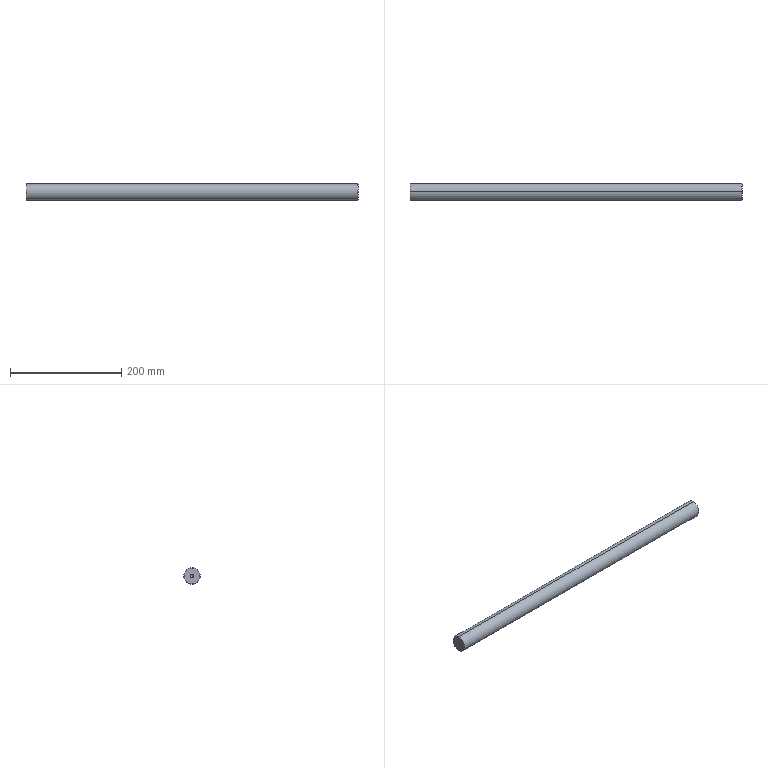Part | STEP file | 001-004-SCD11_D30_L598_M6 | 1 solid | 14 faces | box 598 x 30 x 30 mm | volume 422409 mm3 | cone 8 | cylinder 4 | plane 2 | commonest cylinder face diameters 4.917 x2 30 x2
STEP:
#1=CARTESIAN_POINT('',(0.,0.,0.));
#2=DIRECTION('',(0.,0.,1.));
#3=DIRECTION('',(1.,0.,0.));
#4=AXIS2_PLACEMENT_3D('',#1,#2,#3);
#5=CARTESIAN_POINT('',(598.,0.,14.293));
#6=VERTEX_POINT('',#5);
#7=CARTESIAN_POINT('',(598.,0.,-14.293));
#8=VERTEX_POINT('',#7);
#9=CARTESIAN_POINT('',(598.,0.,0.));
#10=DIRECTION('',(-1.,0.,0.));
#11=DIRECTION('',(0.,0.,1.));
#12=AXIS2_PLACEMENT_3D('',#9,#10,#11);
#13=CIRCLE('',#12,14.293);
#14=CARTESIAN_POINT('',(598.,0.,0.));
#15=DIRECTION('',(-1.,0.,0.));
#16=DIRECTION('',(0.,0.,1.));
#17=AXIS2_PLACEMENT_3D('',#14,#15,#16);
#18=CONICAL_SURFACE('',#17,14.293,0.7854);
#19=CARTESIAN_POINT('',(0.,0.));
#20=DIRECTION('',(1.,0.));
#21=VECTOR('',#20,1.);
#22=LINE('',#19,#21);
#23=(GEOMETRIC_REPRESENTATION_CONTEXT(2)PARAMETRIC_REPRESENTATION_CONTEXT()REPRESENTATION_CONTEXT('',''));
#24=DEFINITIONAL_REPRESENTATION('',(#22),#23);
#25=PCURVE('',#18,#24);
#26=CARTESIAN_POINT('',(598.,14.293,0.));
#27=DIRECTION('',(-1.,0.,0.));
#28=DIRECTION('',(0.,0.,1.));
#29=AXIS2_PLACEMENT_3D('',#26,#27,#28);
#30=PLANE('',#29);
#31=CARTESIAN_POINT('',(0.,-14.293));
#32=DIRECTION('',(1.,0.));
#33=AXIS2_PLACEMENT_2D('',#31,#32);
#34=CIRCLE('',#33,14.293);
#35=(GEOMETRIC_REPRESENTATION_CONTEXT(2)PARAMETRIC_REPRESENTATION_CONTEXT()REPRESENTATION_CONTEXT('',''));
#36=DEFINITIONAL_REPRESENTATION('',(#34),#35);
#37=PCURVE('',#30,#36);
#38=SURFACE_CURVE('',#13,(#25,#37),.PCURVE_S1.);
#39=EDGE_CURVE('',#6,#8,#38,.T.);
#40=ORIENTED_EDGE('',*,*,#39,.T.);
#41=CARTESIAN_POINT('',(597.293,0.,-15.));
#42=VERTEX_POINT('',#41);
#43=CARTESIAN_POINT('',(598.,0.,-14.293));
#44=DIRECTION('',(-0.7071,0.,-0.7071));
#45=VECTOR('',#44,1.);
#46=LINE('',#43,#45);
#47=CARTESIAN_POINT('',(3.142,0.));
#48=DIRECTION('',(0.,1.));
#49=VECTOR('',#48,1.);
#50=LINE('',#47,#49);
#51=(GEOMETRIC_REPRESENTATION_CONTEXT(2)PARAMETRIC_REPRESENTATION_CONTEXT()REPRESENTATION_CONTEXT('',''));
#52=DEFINITIONAL_REPRESENTATION('',(#50),#51);
#53=PCURVE('',#18,#52);
#54=CARTESIAN_POINT('',(598.,0.,0.));
#55=DIRECTION('',(-1.,0.,0.));
#56=DIRECTION('',(0.,0.,1.));
#57=AXIS2_PLACEMENT_3D('',#54,#55,#56);
#58=CONICAL_SURFACE('',#57,14.293,0.7854);
#59=CARTESIAN_POINT('',(3.142,0.));
#60=DIRECTION('',(0.,1.));
#61=VECTOR('',#60,1.);
#62=LINE('',#59,#61);
#63=(GEOMETRIC_REPRESENTATION_CONTEXT(2)PARAMETRIC_REPRESENTATION_CONTEXT()REPRESENTATION_CONTEXT('',''));
#64=DEFINITIONAL_REPRESENTATION('',(#62),#63);
#65=PCURVE('',#58,#64);
#66=SURFACE_CURVE('',#46,(#53,#65),.PCURVE_S1.);
#67=EDGE_CURVE('',#8,#42,#66,.T.);
#68=ORIENTED_EDGE('',*,*,#67,.T.);
#69=CARTESIAN_POINT('',(597.293,0.,15.));
#70=VERTEX_POINT('',#69);
#71=CARTESIAN_POINT('',(597.293,0.,0.));
#72=DIRECTION('',(-1.,0.,0.));
#73=DIRECTION('',(0.,0.,1.));
#74=AXIS2_PLACEMENT_3D('',#71,#72,#73);
#75=CIRCLE('',#74,15.);
#76=CARTESIAN_POINT('',(0.,0.7071));
#77=DIRECTION('',(1.,0.));
#78=VECTOR('',#77,1.);
#79=LINE('',#76,#78);
#80=(GEOMETRIC_REPRESENTATION_CONTEXT(2)PARAMETRIC_REPRESENTATION_CONTEXT()REPRESENTATION_CONTEXT('',''));
#81=DEFINITIONAL_REPRESENTATION('',(#79),#80);
#82=PCURVE('',#18,#81);
#83=CARTESIAN_POINT('',(598.,0.,0.));
#84=DIRECTION('',(-1.,0.,0.));
#85=DIRECTION('',(0.,0.,1.));
#86=AXIS2_PLACEMENT_3D('',#83,#84,#85);
#87=CYLINDRICAL_SURFACE('',#86,15.);
#88=CARTESIAN_POINT('',(0.,0.7071));
#89=DIRECTION('',(1.,0.));
#90=VECTOR('',#89,1.);
#91=LINE('',#88,#90);
#92=(GEOMETRIC_REPRESENTATION_CONTEXT(2)PARAMETRIC_REPRESENTATION_CONTEXT()REPRESENTATION_CONTEXT('',''));
#93=DEFINITIONAL_REPRESENTATION('',(#91),#92);
#94=PCURVE('',#87,#93);
#95=SURFACE_CURVE('',#75,(#82,#94),.PCURVE_S1.);
#96=EDGE_CURVE('',#70,#42,#95,.T.);
#97=ORIENTED_EDGE('',*,*,#96,.F.);
#98=CARTESIAN_POINT('',(598.,0.,14.293));
#99=DIRECTION('',(-0.7071,0.,0.7071));
#100=VECTOR('',#99,1.);
#101=LINE('',#98,#100);
#102=CARTESIAN_POINT('',(0.,0.));
#103=DIRECTION('',(0.,1.));
#104=VECTOR('',#103,1.);
#105=LINE('',#102,#104);
#106=(GEOMETRIC_REPRESENTATION_CONTEXT(2)PARAMETRIC_REPRESENTATION_CONTEXT()REPRESENTATION_CONTEXT('',''));
#107=DEFINITIONAL_REPRESENTATION('',(#105),#106);
#108=PCURVE('',#18,#107);
#109=CARTESIAN_POINT('',(6.283,0.));
#110=DIRECTION('',(0.,1.));
#111=VECTOR('',#110,1.);
#112=LINE('',#109,#111);
#113=(GEOMETRIC_REPRESENTATION_CONTEXT(2)PARAMETRIC_REPRESENTATION_CONTEXT()REPRESENTATION_CONTEXT('',''));
#114=DEFINITIONAL_REPRESENTATION('',(#112),#113);
#115=PCURVE('',#58,#114);
#116=SURFACE_CURVE('',#101,(#108,#115),.PCURVE_S1.);
#117=EDGE_CURVE('',#6,#70,#116,.T.);
#118=ORIENTED_EDGE('',*,*,#117,.F.);
#119=EDGE_LOOP('',(#40,#68,#97,#118));
#120=FACE_BOUND('',#119,.T.);
#121=ADVANCED_FACE('',(#120),#18,.T.);
#122=ORIENTED_EDGE('',*,*,#96,.T.);
#123=CARTESIAN_POINT('',(0.7071,0.,-15.));
#124=VERTEX_POINT('',#123);
#125=CARTESIAN_POINT('',(598.,0.,-15.));
#126=DIRECTION('',(-1.,0.,0.));
#127=VECTOR('',#126,1.);
#128=LINE('',#125,#127);
#129=CARTESIAN_POINT('',(3.142,0.));
#130=DIRECTION('',(0.,1.));
#131=VECTOR('',#130,1.);
#132=LINE('',#129,#131);
#133=(GEOMETRIC_REPRESENTATION_CONTEXT(2)PARAMETRIC_REPRESENTATION_CONTEXT()REPRESENTATION_CONTEXT('',''));
#134=DEFINITIONAL_REPRESENTATION('',(#132),#133);
#135=PCURVE('',#87,#134);
#136=CARTESIAN_POINT('',(598.,0.,0.));
#137=DIRECTION('',(-1.,0.,0.));
#138=DIRECTION('',(0.,0.,1.));
#139=AXIS2_PLACEMENT_3D('',#136,#137,#138);
#140=CYLINDRICAL_SURFACE('',#139,15.);
#141=CARTESIAN_POINT('',(3.142,0.));
#142=DIRECTION('',(0.,1.));
#143=VECTOR('',#142,1.);
#144=LINE('',#141,#143);
#145=(GEOMETRIC_REPRESENTATION_CONTEXT(2)PARAMETRIC_REPRESENTATION_CONTEXT()REPRESENTATION_CONTEXT('',''));
#146=DEFINITIONAL_REPRESENTATION('',(#144),#145);
#147=PCURVE('',#140,#146);
#148=SURFACE_CURVE('',#128,(#135,#147),.PCURVE_S1.);
#149=EDGE_CURVE('',#42,#124,#148,.T.);
#150=ORIENTED_EDGE('',*,*,#149,.T.);
#151=CARTESIAN_POINT('',(0.7071,0.,15.));
#152=VERTEX_POINT('',#151);
#153=CARTESIAN_POINT('',(0.7071,0.,0.));
#154=DIRECTION('',(-1.,0.,0.));
#155=DIRECTION('',(0.,0.,1.));
#156=AXIS2_PLACEMENT_3D('',#153,#154,#155);
#157=CIRCLE('',#156,15.);
#158=CARTESIAN_POINT('',(0.,597.293));
#159=DIRECTION('',(1.,0.));
#160=VECTOR('',#159,1.);
#161=LINE('',#158,#160);
#162=(GEOMETRIC_REPRESENTATION_CONTEXT(2)PARAMETRIC_REPRESENTATION_CONTEXT()REPRESENTATION_CONTEXT('',''));
#163=DEFINITIONAL_REPRESENTATION('',(#161),#162);
#164=PCURVE('',#87,#163);
#165=CARTESIAN_POINT('',(0.7071,0.,0.));
#166=DIRECTION('',(1.,0.,0.));
#167=DIRECTION('',(0.,0.,-1.));
#168=AXIS2_PLACEMENT_3D('',#165,#166,#167);
#169=CONICAL_SURFACE('',#168,15.,0.7854);
#170=CARTESIAN_POINT('',(3.142,0.));
#171=DIRECTION('',(-1.,0.));
#172=VECTOR('',#171,1.);
#173=LINE('',#170,#172);
#174=(GEOMETRIC_REPRESENTATION_CONTEXT(2)PARAMETRIC_REPRESENTATION_CONTEXT()REPRESENTATION_CONTEXT('',''));
#175=DEFINITIONAL_REPRESENTATION('',(#173),#174);
#176=PCURVE('',#169,#175);
#177=SURFACE_CURVE('',#157,(#164,#176),.PCURVE_S1.);
#178=EDGE_CURVE('',#152,#124,#177,.T.);
#179=ORIENTED_EDGE('',*,*,#178,.F.);
#180=CARTESIAN_POINT('',(598.,0.,15.));
#181=DIRECTION('',(-1.,0.,0.));
#182=VECTOR('',#181,1.);
#183=LINE('',#180,#182);
#184=CARTESIAN_POINT('',(0.,0.));
#185=DIRECTION('',(0.,1.));
#186=VECTOR('',#185,1.);
#187=LINE('',#184,#186);
#188=(GEOMETRIC_REPRESENTATION_CONTEXT(2)PARAMETRIC_REPRESENTATION_CONTEXT()REPRESENTATION_CONTEXT('',''));
#189=DEFINITIONAL_REPRESENTATION('',(#187),#188);
#190=PCURVE('',#87,#189);
#191=CARTESIAN_POINT('',(6.283,0.));
#192=DIRECTION('',(0.,1.));
#193=VECTOR('',#192,1.);
#194=LINE('',#191,#193);
#195=(GEOMETRIC_REPRESENTATION_CONTEXT(2)PARAMETRIC_REPRESENTATION_CONTEXT()REPRESENTATION_CONTEXT('',''));
#196=DEFINITIONAL_REPRESENTATION('',(#194),#195);
#197=PCURVE('',#140,#196);
#198=SURFACE_CURVE('',#183,(#190,#197),.PCURVE_S1.);
#199=EDGE_CURVE('',#70,#152,#198,.T.);
#200=ORIENTED_EDGE('',*,*,#199,.F.);
#201=EDGE_LOOP('',(#122,#150,#179,#200));
#202=FACE_BOUND('',#201,.T.);
#203=ADVANCED_FACE('',(#202),#87,.T.);
#204=CARTESIAN_POINT('',(0.,0.,14.293));
#205=VERTEX_POINT('',#204);
#206=CARTESIAN_POINT('',(0.,0.,-14.293));
#207=VERTEX_POINT('',#206);
#208=CARTESIAN_POINT('',(0.,0.,0.));
#209=DIRECTION('',(-1.,0.,0.));
#210=DIRECTION('',(0.,0.,1.));
#211=AXIS2_PLACEMENT_3D('',#208,#209,#210);
#212=CIRCLE('',#211,14.293);
#213=CARTESIAN_POINT('',(3.142,-0.7071));
#214=DIRECTION('',(-1.,0.));
#215=VECTOR('',#214,1.);
#216=LINE('',#213,#215);
#217=(GEOMETRIC_REPRESENTATION_CONTEXT(2)PARAMETRIC_REPRESENTATION_CONTEXT()REPRESENTATION_CONTEXT('',''));
#218=DEFINITIONAL_REPRESENTATION('',(#216),#217);
#219=PCURVE('',#169,#218);
#220=CARTESIAN_POINT('',(0.,3.,0.));
#221=DIRECTION('',(1.,0.,0.));
#222=DIRECTION('',(0.,0.,-1.));
#223=AXIS2_PLACEMENT_3D('',#220,#221,#222);
#224=PLANE('',#223);
#225=CARTESIAN_POINT('',(-14.293,-3.));
#226=CARTESIAN_POINT('',(-14.293,21.756));
#227=CARTESIAN_POINT('',(7.146,9.378));
#228=CARTESIAN_POINT('',(28.586,-3.));
#229=CARTESIAN_POINT('',(7.146,-15.378));
#230=CARTESIAN_POINT('',(-14.293,-27.756));
#231=CARTESIAN_POINT('',(-14.293,-3.));
#232=(BOUNDED_CURVE()B_SPLINE_CURVE(2,(#225,#226,#227,#228,#229,#230,#231),.UNSPECIFIED.,.T.,.F.)B_SPLINE_CURVE_WITH_KNOTS((1,2,2,2,2,1),(-2.094,0.,2.094,4.189,6.283,8.378),.UNSPECIFIED.)CURVE()GEOMETRIC_REPRESENTATION_ITEM()RATIONAL_B_SPLINE_CURVE((1.,0.5,1.,0.5,1.,0.5,1.))REPRESENTATION_ITEM(''));
#233=(GEOMETRIC_REPRESENTATION_CONTEXT(2)PARAMETRIC_REPRESENTATION_CONTEXT()REPRESENTATION_CONTEXT('',''));
#234=DEFINITIONAL_REPRESENTATION('',(#232),#233);
#235=PCURVE('',#224,#234);
#236=SURFACE_CURVE('',#212,(#219,#235),.PCURVE_S1.);
#237=EDGE_CURVE('',#205,#207,#236,.T.);
#238=ORIENTED_EDGE('',*,*,#237,.F.);
#239=CARTESIAN_POINT('',(0.7071,0.,15.));
#240=DIRECTION('',(0.7071,0.,0.7071));
#241=VECTOR('',#240,1.);
#242=LINE('',#239,#241);
#243=CARTESIAN_POINT('',(3.142,0.));
#244=DIRECTION('',(0.,1.));
#245=VECTOR('',#244,1.);
#246=LINE('',#243,#245);
#247=(GEOMETRIC_REPRESENTATION_CONTEXT(2)PARAMETRIC_REPRESENTATION_CONTEXT()REPRESENTATION_CONTEXT('',''));
#248=DEFINITIONAL_REPRESENTATION('',(#246),#247);
#249=PCURVE('',#169,#248);
#250=CARTESIAN_POINT('',(0.7071,0.,0.));
#251=DIRECTION('',(1.,0.,0.));
#252=DIRECTION('',(0.,0.,-1.));
#253=AXIS2_PLACEMENT_3D('',#250,#251,#252);
#254=CONICAL_SURFACE('',#253,15.,0.7854);
#255=CARTESIAN_POINT('',(3.142,0.));
#256=DIRECTION('',(0.,1.));
#257=VECTOR('',#256,1.);
#258=LINE('',#255,#257);
#259=(GEOMETRIC_REPRESENTATION_CONTEXT(2)PARAMETRIC_REPRESENTATION_CONTEXT()REPRESENTATION_CONTEXT('',''));
#260=DEFINITIONAL_REPRESENTATION('',(#258),#259);
#261=PCURVE('',#254,#260);
#262=SURFACE_CURVE('',#242,(#249,#261),.PCURVE_S1.);
#263=EDGE_CURVE('',#205,#152,#262,.T.);
#264=ORIENTED_EDGE('',*,*,#263,.T.);
#265=ORIENTED_EDGE('',*,*,#178,.T.);
#266=CARTESIAN_POINT('',(0.7071,0.,-15.));
#267=DIRECTION('',(0.7071,0.,-0.7071));
#268=VECTOR('',#267,1.);
#269=LINE('',#266,#268);
#270=CARTESIAN_POINT('',(0.,0.));
#271=DIRECTION('',(0.,1.));
#272=VECTOR('',#271,1.);
#273=LINE('',#270,#272);
#274=(GEOMETRIC_REPRESENTATION_CONTEXT(2)PARAMETRIC_REPRESENTATION_CONTEXT()REPRESENTATION_CONTEXT('',''));
#275=DEFINITIONAL_REPRESENTATION('',(#273),#274);
#276=PCURVE('',#169,#275);
#277=CARTESIAN_POINT('',(6.283,0.));
#278=DIRECTION('',(0.,1.));
#279=VECTOR('',#278,1.);
#280=LINE('',#277,#279);
#281=(GEOMETRIC_REPRESENTATION_CONTEXT(2)PARAMETRIC_REPRESENTATION_CONTEXT()REPRESENTATION_CONTEXT('',''));
#282=DEFINITIONAL_REPRESENTATION('',(#280),#281);
#283=PCURVE('',#254,#282);
#284=SURFACE_CURVE('',#269,(#276,#283),.PCURVE_S1.);
#285=EDGE_CURVE('',#207,#124,#284,.T.);
#286=ORIENTED_EDGE('',*,*,#285,.F.);
#287=EDGE_LOOP('',(#238,#264,#265,#286));
#288=FACE_BOUND('',#287,.T.);
#289=ADVANCED_FACE('',(#288),#169,.T.);
#290=CARTESIAN_POINT('',(0.5415,0.,2.458));
#291=VERTEX_POINT('',#290);
#292=CARTESIAN_POINT('',(0.,0.,3.));
#293=VERTEX_POINT('',#292);
#294=CARTESIAN_POINT('',(0.,0.,3.));
#295=DIRECTION('',(-0.7071,0.,0.7071));
#296=VECTOR('',#295,1.);
#297=LINE('',#294,#296);
#298=CARTESIAN_POINT('',(0.,0.,0.));
#299=DIRECTION('',(-1.,0.,0.));
#300=DIRECTION('',(0.,0.,1.));
#301=AXIS2_PLACEMENT_3D('',#298,#299,#300);
#302=CONICAL_SURFACE('',#301,3.,0.7854);
#303=CARTESIAN_POINT('',(6.283,0.));
#304=DIRECTION('',(0.,1.));
#305=VECTOR('',#304,1.);
#306=LINE('',#303,#305);
#307=(GEOMETRIC_REPRESENTATION_CONTEXT(2)PARAMETRIC_REPRESENTATION_CONTEXT()REPRESENTATION_CONTEXT('',''));
#308=DEFINITIONAL_REPRESENTATION('',(#306),#307);
#309=PCURVE('',#302,#308);
#310=CARTESIAN_POINT('',(0.,0.,0.));
#311=DIRECTION('',(-1.,0.,0.));
#312=DIRECTION('',(0.,0.,1.));
#313=AXIS2_PLACEMENT_3D('',#310,#311,#312);
#314=CONICAL_SURFACE('',#313,3.,0.7854);
#315=CARTESIAN_POINT('',(0.,0.));
#316=DIRECTION('',(0.,1.));
#317=VECTOR('',#316,1.);
#318=LINE('',#315,#317);
#319=(GEOMETRIC_REPRESENTATION_CONTEXT(2)PARAMETRIC_REPRESENTATION_CONTEXT()REPRESENTATION_CONTEXT('',''));
#320=DEFINITIONAL_REPRESENTATION('',(#318),#319);
#321=PCURVE('',#314,#320);
#322=SURFACE_CURVE('',#297,(#309,#321),.PCURVE_S1.);
#323=EDGE_CURVE('',#291,#293,#322,.T.);
#324=ORIENTED_EDGE('',*,*,#323,.T.);
#325=CARTESIAN_POINT('',(0.,0.,-3.));
#326=VERTEX_POINT('',#325);
#327=CARTESIAN_POINT('',(0.,0.,0.));
#328=DIRECTION('',(-1.,0.,0.));
#329=DIRECTION('',(0.,0.,1.));
#330=AXIS2_PLACEMENT_3D('',#327,#328,#329);
#331=CIRCLE('',#330,3.);
#332=CARTESIAN_POINT('',(0.,0.));
#333=DIRECTION('',(1.,0.));
#334=VECTOR('',#333,1.);
#335=LINE('',#332,#334);
#336=(GEOMETRIC_REPRESENTATION_CONTEXT(2)PARAMETRIC_REPRESENTATION_CONTEXT()REPRESENTATION_CONTEXT('',''));
#337=DEFINITIONAL_REPRESENTATION('',(#335),#336);
#338=PCURVE('',#302,#337);
#339=CARTESIAN_POINT('',(-3.,-3.));
#340=CARTESIAN_POINT('',(-3.,2.196));
#341=CARTESIAN_POINT('',(1.5,-0.4019));
#342=CARTESIAN_POINT('',(6.,-3.));
#343=CARTESIAN_POINT('',(1.5,-5.598));
#344=CARTESIAN_POINT('',(-3.,-8.196));
#345=CARTESIAN_POINT('',(-3.,-3.));
#346=(BOUNDED_CURVE()B_SPLINE_CURVE(2,(#339,#340,#341,#342,#343,#344,#345),.UNSPECIFIED.,.T.,.F.)B_SPLINE_CURVE_WITH_KNOTS((1,2,2,2,2,1),(-2.094,0.,2.094,4.189,6.283,8.378),.UNSPECIFIED.)CURVE()GEOMETRIC_REPRESENTATION_ITEM()RATIONAL_B_SPLINE_CURVE((1.,0.5,1.,0.5,1.,0.5,1.))REPRESENTATION_ITEM(''));
#347=(GEOMETRIC_REPRESENTATION_CONTEXT(2)PARAMETRIC_REPRESENTATION_CONTEXT()REPRESENTATION_CONTEXT('',''));
#348=DEFINITIONAL_REPRESENTATION('',(#346),#347);
#349=PCURVE('',#224,#348);
#350=SURFACE_CURVE('',#331,(#338,#349),.PCURVE_S1.);
#351=EDGE_CURVE('',#326,#293,#350,.T.);
#352=ORIENTED_EDGE('',*,*,#351,.F.);
#353=CARTESIAN_POINT('',(0.5415,0.,-2.458));
#354=VERTEX_POINT('',#353);
#355=CARTESIAN_POINT('',(0.,0.,-3.));
#356=DIRECTION('',(-0.7071,0.,-0.7071));
#357=VECTOR('',#356,1.);
#358=LINE('',#355,#357);
#359=CARTESIAN_POINT('',(3.142,0.));
#360=DIRECTION('',(0.,1.));
#361=VECTOR('',#360,1.);
#362=LINE('',#359,#361);
#363=(GEOMETRIC_REPRESENTATION_CONTEXT(2)PARAMETRIC_REPRESENTATION_CONTEXT()REPRESENTATION_CONTEXT('',''));
#364=DEFINITIONAL_REPRESENTATION('',(#362),#363);
#365=PCURVE('',#302,#364);
#366=CARTESIAN_POINT('',(3.142,0.));
#367=DIRECTION('',(0.,1.));
#368=VECTOR('',#367,1.);
#369=LINE('',#366,#368);
#370=(GEOMETRIC_REPRESENTATION_CONTEXT(2)PARAMETRIC_REPRESENTATION_CONTEXT()REPRESENTATION_CONTEXT('',''));
#371=DEFINITIONAL_REPRESENTATION('',(#369),#370);
#372=PCURVE('',#314,#371);
#373=SURFACE_CURVE('',#358,(#365,#372),.PCURVE_S1.);
#374=EDGE_CURVE('',#354,#326,#373,.T.);
#375=ORIENTED_EDGE('',*,*,#374,.F.);
#376=CARTESIAN_POINT('',(0.5415,0.,0.));
#377=DIRECTION('',(-1.,0.,0.));
#378=DIRECTION('',(0.,0.,1.));
#379=AXIS2_PLACEMENT_3D('',#376,#377,#378);
#380=CIRCLE('',#379,2.458);
#381=CARTESIAN_POINT('',(0.,-0.5415));
#382=DIRECTION('',(1.,0.));
#383=VECTOR('',#382,1.);
#384=LINE('',#381,#383);
#385=(GEOMETRIC_REPRESENTATION_CONTEXT(2)PARAMETRIC_REPRESENTATION_CONTEXT()REPRESENTATION_CONTEXT('',''));
#386=DEFINITIONAL_REPRESENTATION('',(#384),#385);
#387=PCURVE('',#302,#386);
#388=CARTESIAN_POINT('',(598.,0.,0.));
#389=DIRECTION('',(-1.,0.,0.));
#390=DIRECTION('',(0.,0.,1.));
#391=AXIS2_PLACEMENT_3D('',#388,#389,#390);
#392=CYLINDRICAL_SURFACE('',#391,2.458);
#393=CARTESIAN_POINT('',(0.,597.458));
#394=DIRECTION('',(1.,0.));
#395=VECTOR('',#394,1.);
#396=LINE('',#393,#395);
#397=(GEOMETRIC_REPRESENTATION_CONTEXT(2)PARAMETRIC_REPRESENTATION_CONTEXT()REPRESENTATION_CONTEXT('',''));
#398=DEFINITIONAL_REPRESENTATION('',(#396),#397);
#399=PCURVE('',#392,#398);
#400=SURFACE_CURVE('',#380,(#387,#399),.PCURVE_S1.);
#401=EDGE_CURVE('',#354,#291,#400,.T.);
#402=ORIENTED_EDGE('',*,*,#401,.T.);
#403=EDGE_LOOP('',(#324,#352,#375,#402));
#404=FACE_BOUND('',#403,.F.);
#405=ADVANCED_FACE('',(#404),#302,.F.);
#406=CARTESIAN_POINT('',(12.325,0.,2.458));
#407=VERTEX_POINT('',#406);
#408=CARTESIAN_POINT('',(598.,0.,2.458));
#409=DIRECTION('',(-1.,0.,0.));
#410=VECTOR('',#409,1.);
#411=LINE('',#408,#410);
#412=CARTESIAN_POINT('',(6.283,0.));
#413=DIRECTION('',(0.,1.));
#414=VECTOR('',#413,1.);
#415=LINE('',#412,#414);
#416=(GEOMETRIC_REPRESENTATION_CONTEXT(2)PARAMETRIC_REPRESENTATION_CONTEXT()REPRESENTATION_CONTEXT('',''));
#417=DEFINITIONAL_REPRESENTATION('',(#415),#416);
#418=PCURVE('',#392,#417);
#419=CARTESIAN_POINT('',(598.,0.,0.));
#420=DIRECTION('',(-1.,0.,0.));
#421=DIRECTION('',(0.,0.,1.));
#422=AXIS2_PLACEMENT_3D('',#419,#420,#421);
#423=CYLINDRICAL_SURFACE('',#422,2.458);
#424=CARTESIAN_POINT('',(0.,0.));
#425=DIRECTION('',(0.,1.));
#426=VECTOR('',#425,1.);
#427=LINE('',#424,#426);
#428=(GEOMETRIC_REPRESENTATION_CONTEXT(2)PARAMETRIC_REPRESENTATION_CONTEXT()REPRESENTATION_CONTEXT('',''));
#429=DEFINITIONAL_REPRESENTATION('',(#427),#428);
#430=PCURVE('',#423,#429);
#431=SURFACE_CURVE('',#411,(#418,#430),.PCURVE_S1.);
#432=EDGE_CURVE('',#407,#291,#431,.T.);
#433=ORIENTED_EDGE('',*,*,#432,.T.);
#434=ORIENTED_EDGE('',*,*,#401,.F.);
#435=CARTESIAN_POINT('',(12.325,0.,-2.458));
#436=VERTEX_POINT('',#435);
#437=CARTESIAN_POINT('',(598.,0.,-2.458));
#438=DIRECTION('',(-1.,0.,0.));
#439=VECTOR('',#438,1.);
#440=LINE('',#437,#439);
#441=CARTESIAN_POINT('',(3.142,0.));
#442=DIRECTION('',(0.,1.));
#443=VECTOR('',#442,1.);
#444=LINE('',#441,#443);
#445=(GEOMETRIC_REPRESENTATION_CONTEXT(2)PARAMETRIC_REPRESENTATION_CONTEXT()REPRESENTATION_CONTEXT('',''));
#446=DEFINITIONAL_REPRESENTATION('',(#444),#445);
#447=PCURVE('',#392,#446);
#448=CARTESIAN_POINT('',(3.142,0.));
#449=DIRECTION('',(0.,1.));
#450=VECTOR('',#449,1.);
#451=LINE('',#448,#450);
#452=(GEOMETRIC_REPRESENTATION_CONTEXT(2)PARAMETRIC_REPRESENTATION_CONTEXT()REPRESENTATION_CONTEXT('',''));
#453=DEFINITIONAL_REPRESENTATION('',(#451),#452);
#454=PCURVE('',#423,#453);
#455=SURFACE_CURVE('',#440,(#447,#454),.PCURVE_S1.);
#456=EDGE_CURVE('',#436,#354,#455,.T.);
#457=ORIENTED_EDGE('',*,*,#456,.F.);
#458=CARTESIAN_POINT('',(12.325,0.,0.));
#459=DIRECTION('',(-1.,0.,0.));
#460=DIRECTION('',(0.,0.,1.));
#461=AXIS2_PLACEMENT_3D('',#458,#459,#460);
#462=CIRCLE('',#461,2.458);
#463=CARTESIAN_POINT('',(0.,585.675));
#464=DIRECTION('',(1.,0.));
#465=VECTOR('',#464,1.);
#466=LINE('',#463,#465);
#467=(GEOMETRIC_REPRESENTATION_CONTEXT(2)PARAMETRIC_REPRESENTATION_CONTEXT()REPRESENTATION_CONTEXT('',''));
#468=DEFINITIONAL_REPRESENTATION('',(#466),#467);
#469=PCURVE('',#392,#468);
#470=CARTESIAN_POINT('',(12.325,0.,0.));
#471=DIRECTION('',(-1.,0.,0.));
#472=DIRECTION('',(0.,0.,1.));
#473=AXIS2_PLACEMENT_3D('',#470,#471,#472);
#474=CONICAL_SURFACE('',#473,2.458,1.03);
#475=CARTESIAN_POINT('',(0.,0.));
#476=DIRECTION('',(1.,0.));
#477=VECTOR('',#476,1.);
#478=LINE('',#475,#477);
#479=(GEOMETRIC_REPRESENTATION_CONTEXT(2)PARAMETRIC_REPRESENTATION_CONTEXT()REPRESENTATION_CONTEXT('',''));
#480=DEFINITIONAL_REPRESENTATION('',(#478),#479);
#481=PCURVE('',#474,#480);
#482=SURFACE_CURVE('',#462,(#469,#481),.PCURVE_S1.);
#483=EDGE_CURVE('',#436,#407,#482,.T.);
#484=ORIENTED_EDGE('',*,*,#483,.T.);
#485=EDGE_LOOP('',(#433,#434,#457,#484));
#486=FACE_BOUND('',#485,.F.);
#487=ADVANCED_FACE('',(#486),#392,.F.);
#488=ORIENTED_EDGE('',*,*,#483,.F.);
#489=CARTESIAN_POINT('',(13.803,0.,0.));
#490=VERTEX_POINT('',#489);
#491=CARTESIAN_POINT('',(12.325,0.,-2.458));
#492=DIRECTION('',(-0.515,0.,-0.8572));
#493=VECTOR('',#492,1.);
#494=LINE('',#491,#493);
#495=CARTESIAN_POINT('',(3.142,0.));
#496=DIRECTION('',(0.,1.));
#497=VECTOR('',#496,1.);
#498=LINE('',#495,#497);
#499=(GEOMETRIC_REPRESENTATION_CONTEXT(2)PARAMETRIC_REPRESENTATION_CONTEXT()REPRESENTATION_CONTEXT('',''));
#500=DEFINITIONAL_REPRESENTATION('',(#498),#499);
#501=PCURVE('',#474,#500);
#502=CARTESIAN_POINT('',(12.325,0.,0.));
#503=DIRECTION('',(-1.,0.,0.));
#504=DIRECTION('',(0.,0.,1.));
#505=AXIS2_PLACEMENT_3D('',#502,#503,#504);
#506=CONICAL_SURFACE('',#505,2.458,1.03);
#507=CARTESIAN_POINT('',(3.142,0.));
#508=DIRECTION('',(0.,1.));
#509=VECTOR('',#508,1.);
#510=LINE('',#507,#509);
#511=(GEOMETRIC_REPRESENTATION_CONTEXT(2)PARAMETRIC_REPRESENTATION_CONTEXT()REPRESENTATION_CONTEXT('',''));
#512=DEFINITIONAL_REPRESENTATION('',(#510),#511);
#513=PCURVE('',#506,#512);
#514=SURFACE_CURVE('',#494,(#501,#513),.PCURVE_S1.);
#515=EDGE_CURVE('',#490,#436,#514,.T.);
#516=ORIENTED_EDGE('',*,*,#515,.F.);
#517=CARTESIAN_POINT('',(12.325,0.,2.458));
#518=DIRECTION('',(-0.515,0.,0.8572));
#519=VECTOR('',#518,1.);
#520=LINE('',#517,#519);
#521=CARTESIAN_POINT('',(6.283,0.));
#522=DIRECTION('',(0.,1.));
#523=VECTOR('',#522,1.);
#524=LINE('',#521,#523);
#525=(GEOMETRIC_REPRESENTATION_CONTEXT(2)PARAMETRIC_REPRESENTATION_CONTEXT()REPRESENTATION_CONTEXT('',''));
#526=DEFINITIONAL_REPRESENTATION('',(#524),#525);
#527=PCURVE('',#474,#526);
#528=CARTESIAN_POINT('',(0.,0.));
#529=DIRECTION('',(0.,1.));
#530=VECTOR('',#529,1.);
#531=LINE('',#528,#530);
#532=(GEOMETRIC_REPRESENTATION_CONTEXT(2)PARAMETRIC_REPRESENTATION_CONTEXT()REPRESENTATION_CONTEXT('',''));
#533=DEFINITIONAL_REPRESENTATION('',(#531),#532);
#534=PCURVE('',#506,#533);
#535=SURFACE_CURVE('',#520,(#527,#534),.PCURVE_S1.);
#536=EDGE_CURVE('',#490,#407,#535,.T.);
#537=ORIENTED_EDGE('',*,*,#536,.T.);
#538=EDGE_LOOP('',(#488,#516,#537));
#539=FACE_BOUND('',#538,.F.);
#540=ADVANCED_FACE('',(#539),#474,.F.);
#541=CARTESIAN_POINT('',(12.325,0.,0.));
#542=DIRECTION('',(-1.,0.,0.));
#543=DIRECTION('',(0.,0.,1.));
#544=AXIS2_PLACEMENT_3D('',#541,#542,#543);
#545=CIRCLE('',#544,2.458);
#546=CARTESIAN_POINT('',(0.,0.));
#547=DIRECTION('',(1.,0.));
#548=VECTOR('',#547,1.);
#549=LINE('',#546,#548);
#550=(GEOMETRIC_REPRESENTATION_CONTEXT(2)PARAMETRIC_REPRESENTATION_CONTEXT()REPRESENTATION_CONTEXT('',''));
#551=DEFINITIONAL_REPRESENTATION('',(#549),#550);
#552=PCURVE('',#506,#551);
#553=CARTESIAN_POINT('',(0.,585.675));
#554=DIRECTION('',(1.,0.));
#555=VECTOR('',#554,1.);
#556=LINE('',#553,#555);
#557=(GEOMETRIC_REPRESENTATION_CONTEXT(2)PARAMETRIC_REPRESENTATION_CONTEXT()REPRESENTATION_CONTEXT('',''));
#558=DEFINITIONAL_REPRESENTATION('',(#556),#557);
#559=PCURVE('',#423,#558);
#560=SURFACE_CURVE('',#545,(#552,#559),.PCURVE_S1.);
#561=EDGE_CURVE('',#407,#436,#560,.T.);
#562=ORIENTED_EDGE('',*,*,#561,.F.);
#563=ORIENTED_EDGE('',*,*,#536,.F.);
#564=ORIENTED_EDGE('',*,*,#515,.T.);
#565=EDGE_LOOP('',(#562,#563,#564));
#566=FACE_BOUND('',#565,.F.);
#567=ADVANCED_FACE('',(#566),#506,.F.);
#568=CARTESIAN_POINT('',(0.5415,0.,0.));
#569=DIRECTION('',(-1.,0.,0.));
#570=DIRECTION('',(0.,0.,1.));
#571=AXIS2_PLACEMENT_3D('',#568,#569,#570);
#572=CIRCLE('',#571,2.458);
#573=CARTESIAN_POINT('',(0.,597.458));
#574=DIRECTION('',(1.,0.));
#575=VECTOR('',#574,1.);
#576=LINE('',#573,#575);
#577=(GEOMETRIC_REPRESENTATION_CONTEXT(2)PARAMETRIC_REPRESENTATION_CONTEXT()REPRESENTATION_CONTEXT('',''));
#578=DEFINITIONAL_REPRESENTATION('',(#576),#577);
#579=PCURVE('',#423,#578);
#580=CARTESIAN_POINT('',(0.,-0.5415));
#581=DIRECTION('',(1.,0.));
#582=VECTOR('',#581,1.);
#583=LINE('',#580,#582);
#584=(GEOMETRIC_REPRESENTATION_CONTEXT(2)PARAMETRIC_REPRESENTATION_CONTEXT()REPRESENTATION_CONTEXT('',''));
#585=DEFINITIONAL_REPRESENTATION('',(#583),#584);
#586=PCURVE('',#314,#585);
#587=SURFACE_CURVE('',#572,(#579,#586),.PCURVE_S1.);
#588=EDGE_CURVE('',#291,#354,#587,.T.);
#589=ORIENTED_EDGE('',*,*,#588,.F.);
#590=ORIENTED_EDGE('',*,*,#432,.F.);
#591=ORIENTED_EDGE('',*,*,#561,.T.);
#592=ORIENTED_EDGE('',*,*,#456,.T.);
#593=EDGE_LOOP('',(#589,#590,#591,#592));
#594=FACE_BOUND('',#593,.F.);
#595=ADVANCED_FACE('',(#594),#423,.F.);
#596=CARTESIAN_POINT('',(0.,0.,0.));
#597=DIRECTION('',(-1.,0.,0.));
#598=DIRECTION('',(0.,0.,1.));
#599=AXIS2_PLACEMENT_3D('',#596,#597,#598);
#600=CIRCLE('',#599,3.);
#601=CARTESIAN_POINT('',(0.,0.));
#602=DIRECTION('',(1.,0.));
#603=VECTOR('',#602,1.);
#604=LINE('',#601,#603);
#605=(GEOMETRIC_REPRESENTATION_CONTEXT(2)PARAMETRIC_REPRESENTATION_CONTEXT()REPRESENTATION_CONTEXT('',''));
#606=DEFINITIONAL_REPRESENTATION('',(#604),#605);
#607=PCURVE('',#314,#606);
#608=CARTESIAN_POINT('',(-3.,-3.));
#609=CARTESIAN_POINT('',(-3.,2.196));
#610=CARTESIAN_POINT('',(1.5,-0.4019));
#611=CARTESIAN_POINT('',(6.,-3.));
#612=CARTESIAN_POINT('',(1.5,-5.598));
#613=CARTESIAN_POINT('',(-3.,-8.196));
#614=CARTESIAN_POINT('',(-3.,-3.));
#615=(BOUNDED_CURVE()B_SPLINE_CURVE(2,(#608,#609,#610,#611,#612,#613,#614),.UNSPECIFIED.,.T.,.F.)B_SPLINE_CURVE_WITH_KNOTS((1,2,2,2,2,1),(-2.094,0.,2.094,4.189,6.283,8.378),.UNSPECIFIED.)CURVE()GEOMETRIC_REPRESENTATION_ITEM()RATIONAL_B_SPLINE_CURVE((1.,0.5,1.,0.5,1.,0.5,1.))REPRESENTATION_ITEM(''));
#616=(GEOMETRIC_REPRESENTATION_CONTEXT(2)PARAMETRIC_REPRESENTATION_CONTEXT()REPRESENTATION_CONTEXT('',''));
#617=DEFINITIONAL_REPRESENTATION('',(#615),#616);
#618=PCURVE('',#224,#617);
#619=SURFACE_CURVE('',#600,(#607,#618),.PCURVE_S1.);
#620=EDGE_CURVE('',#293,#326,#619,.T.);
#621=ORIENTED_EDGE('',*,*,#620,.F.);
#622=ORIENTED_EDGE('',*,*,#323,.F.);
#623=ORIENTED_EDGE('',*,*,#588,.T.);
#624=ORIENTED_EDGE('',*,*,#374,.T.);
#625=EDGE_LOOP('',(#621,#622,#623,#624));
#626=FACE_BOUND('',#625,.F.);
#627=ADVANCED_FACE('',(#626),#314,.F.);
#628=ORIENTED_EDGE('',*,*,#620,.F.);
#629=ORIENTED_EDGE('',*,*,#351,.F.);
#630=EDGE_LOOP('',(#628,#629));
#631=FACE_BOUND('',#630,.T.);
#632=CARTESIAN_POINT('',(0.,0.,0.));
#633=DIRECTION('',(-1.,0.,0.));
#634=DIRECTION('',(0.,0.,1.));
#635=AXIS2_PLACEMENT_3D('',#632,#633,#634);
#636=CIRCLE('',#635,14.293);
#637=CARTESIAN_POINT('',(-14.293,-3.));
#638=CARTESIAN_POINT('',(-14.293,21.756));
#639=CARTESIAN_POINT('',(7.146,9.378));
#640=CARTESIAN_POINT('',(28.586,-3.));
#641=CARTESIAN_POINT('',(7.146,-15.378));
#642=CARTESIAN_POINT('',(-14.293,-27.756));
#643=CARTESIAN_POINT('',(-14.293,-3.));
#644=(BOUNDED_CURVE()B_SPLINE_CURVE(2,(#637,#638,#639,#640,#641,#642,#643),.UNSPECIFIED.,.T.,.F.)B_SPLINE_CURVE_WITH_KNOTS((1,2,2,2,2,1),(-2.094,0.,2.094,4.189,6.283,8.378),.UNSPECIFIED.)CURVE()GEOMETRIC_REPRESENTATION_ITEM()RATIONAL_B_SPLINE_CURVE((1.,0.5,1.,0.5,1.,0.5,1.))REPRESENTATION_ITEM(''));
#645=(GEOMETRIC_REPRESENTATION_CONTEXT(2)PARAMETRIC_REPRESENTATION_CONTEXT()REPRESENTATION_CONTEXT('',''));
#646=DEFINITIONAL_REPRESENTATION('',(#644),#645);
#647=PCURVE('',#224,#646);
#648=CARTESIAN_POINT('',(9.425,-0.7071));
#649=DIRECTION('',(-1.,0.));
#650=VECTOR('',#649,1.);
#651=LINE('',#648,#650);
#652=(GEOMETRIC_REPRESENTATION_CONTEXT(2)PARAMETRIC_REPRESENTATION_CONTEXT()REPRESENTATION_CONTEXT('',''));
#653=DEFINITIONAL_REPRESENTATION('',(#651),#652);
#654=PCURVE('',#254,#653);
#655=SURFACE_CURVE('',#636,(#647,#654),.PCURVE_S1.);
#656=EDGE_CURVE('',#207,#205,#655,.T.);
#657=ORIENTED_EDGE('',*,*,#656,.T.);
#658=ORIENTED_EDGE('',*,*,#237,.T.);
#659=EDGE_LOOP('',(#657,#658));
#660=FACE_BOUND('',#659,.T.);
#661=ADVANCED_FACE('',(#631,#660),#224,.F.);
#662=ORIENTED_EDGE('',*,*,#263,.F.);
#663=ORIENTED_EDGE('',*,*,#656,.F.);
#664=ORIENTED_EDGE('',*,*,#285,.T.);
#665=CARTESIAN_POINT('',(0.7071,0.,0.));
#666=DIRECTION('',(-1.,0.,0.));
#667=DIRECTION('',(0.,0.,1.));
#668=AXIS2_PLACEMENT_3D('',#665,#666,#667);
#669=CIRCLE('',#668,15.);
#670=CARTESIAN_POINT('',(9.425,0.));
#671=DIRECTION('',(-1.,0.));
#672=VECTOR('',#671,1.);
#673=LINE('',#670,#672);
#674=(GEOMETRIC_REPRESENTATION_CONTEXT(2)PARAMETRIC_REPRESENTATION_CONTEXT()REPRESENTATION_CONTEXT('',''));
#675=DEFINITIONAL_REPRESENTATION('',(#673),#674);
#676=PCURVE('',#254,#675);
#677=CARTESIAN_POINT('',(0.,597.293));
#678=DIRECTION('',(1.,0.));
#679=VECTOR('',#678,1.);
#680=LINE('',#677,#679);
#681=(GEOMETRIC_REPRESENTATION_CONTEXT(2)PARAMETRIC_REPRESENTATION_CONTEXT()REPRESENTATION_CONTEXT('',''));
#682=DEFINITIONAL_REPRESENTATION('',(#680),#681);
#683=PCURVE('',#140,#682);
#684=SURFACE_CURVE('',#669,(#676,#683),.PCURVE_S1.);
#685=EDGE_CURVE('',#124,#152,#684,.T.);
#686=ORIENTED_EDGE('',*,*,#685,.T.);
#687=EDGE_LOOP('',(#662,#663,#664,#686));
#688=FACE_BOUND('',#687,.T.);
#689=ADVANCED_FACE('',(#688),#254,.T.);
#690=ORIENTED_EDGE('',*,*,#149,.F.);
#691=CARTESIAN_POINT('',(597.293,0.,0.));
#692=DIRECTION('',(-1.,0.,0.));
#693=DIRECTION('',(0.,0.,1.));
#694=AXIS2_PLACEMENT_3D('',#691,#692,#693);
#695=CIRCLE('',#694,15.);
#696=CARTESIAN_POINT('',(0.,0.7071));
#697=DIRECTION('',(1.,0.));
#698=VECTOR('',#697,1.);
#699=LINE('',#696,#698);
#700=(GEOMETRIC_REPRESENTATION_CONTEXT(2)PARAMETRIC_REPRESENTATION_CONTEXT()REPRESENTATION_CONTEXT('',''));
#701=DEFINITIONAL_REPRESENTATION('',(#699),#700);
#702=PCURVE('',#140,#701);
#703=CARTESIAN_POINT('',(0.,0.7071));
#704=DIRECTION('',(1.,0.));
#705=VECTOR('',#704,1.);
#706=LINE('',#703,#705);
#707=(GEOMETRIC_REPRESENTATION_CONTEXT(2)PARAMETRIC_REPRESENTATION_CONTEXT()REPRESENTATION_CONTEXT('',''));
#708=DEFINITIONAL_REPRESENTATION('',(#706),#707);
#709=PCURVE('',#58,#708);
#710=SURFACE_CURVE('',#695,(#702,#709),.PCURVE_S1.);
#711=EDGE_CURVE('',#42,#70,#710,.T.);
#712=ORIENTED_EDGE('',*,*,#711,.T.);
#713=ORIENTED_EDGE('',*,*,#199,.T.);
#714=ORIENTED_EDGE('',*,*,#685,.F.);
#715=EDGE_LOOP('',(#690,#712,#713,#714));
#716=FACE_BOUND('',#715,.T.);
#717=ADVANCED_FACE('',(#716),#140,.T.);
#718=ORIENTED_EDGE('',*,*,#67,.F.);
#719=CARTESIAN_POINT('',(598.,0.,0.));
#720=DIRECTION('',(-1.,0.,0.));
#721=DIRECTION('',(0.,0.,1.));
#722=AXIS2_PLACEMENT_3D('',#719,#720,#721);
#723=CIRCLE('',#722,14.293);
#724=CARTESIAN_POINT('',(0.,0.));
#725=DIRECTION('',(1.,0.));
#726=VECTOR('',#725,1.);
#727=LINE('',#724,#726);
#728=(GEOMETRIC_REPRESENTATION_CONTEXT(2)PARAMETRIC_REPRESENTATION_CONTEXT()REPRESENTATION_CONTEXT('',''));
#729=DEFINITIONAL_REPRESENTATION('',(#727),#728);
#730=PCURVE('',#58,#729);
#731=CARTESIAN_POINT('',(0.,-14.293));
#732=DIRECTION('',(1.,0.));
#733=AXIS2_PLACEMENT_2D('',#731,#732);
#734=CIRCLE('',#733,14.293);
#735=(GEOMETRIC_REPRESENTATION_CONTEXT(2)PARAMETRIC_REPRESENTATION_CONTEXT()REPRESENTATION_CONTEXT('',''));
#736=DEFINITIONAL_REPRESENTATION('',(#734),#735);
#737=PCURVE('',#30,#736);
#738=SURFACE_CURVE('',#723,(#730,#737),.PCURVE_S1.);
#739=EDGE_CURVE('',#8,#6,#738,.T.);
#740=ORIENTED_EDGE('',*,*,#739,.T.);
#741=ORIENTED_EDGE('',*,*,#117,.T.);
#742=ORIENTED_EDGE('',*,*,#711,.F.);
#743=EDGE_LOOP('',(#718,#740,#741,#742));
#744=FACE_BOUND('',#743,.T.);
#745=ADVANCED_FACE('',(#744),#58,.T.);
#746=ORIENTED_EDGE('',*,*,#39,.F.);
#747=ORIENTED_EDGE('',*,*,#739,.F.);
#748=EDGE_LOOP('',(#746,#747));
#749=FACE_BOUND('',#748,.T.);
#750=ADVANCED_FACE('',(#749),#30,.F.);
#751=CLOSED_SHELL('',(#121,#203,#289,#405,#487,#540,#567,#595,#627,#661,#689,#717,#745,#750));
#752=MANIFOLD_SOLID_BREP('',#751);
#753=(LENGTH_UNIT()NAMED_UNIT(*)SI_UNIT(.MILLI.,.METRE.));
#754=UNCERTAINTY_MEASURE_WITH_UNIT(LENGTH_MEASURE(0.0000001),#753,'','');
#755=(NAMED_UNIT(*)PLANE_ANGLE_UNIT()SI_UNIT($,.RADIAN.));
#756=(NAMED_UNIT(*)SI_UNIT($,.STERADIAN.)SOLID_ANGLE_UNIT());
#757=(GEOMETRIC_REPRESENTATION_CONTEXT(3)GLOBAL_UNCERTAINTY_ASSIGNED_CONTEXT((#754))GLOBAL_UNIT_ASSIGNED_CONTEXT((#753,#755,#756))REPRESENTATION_CONTEXT('',''));
#758=ADVANCED_BREP_SHAPE_REPRESENTATION('',(#4,#752),#757);